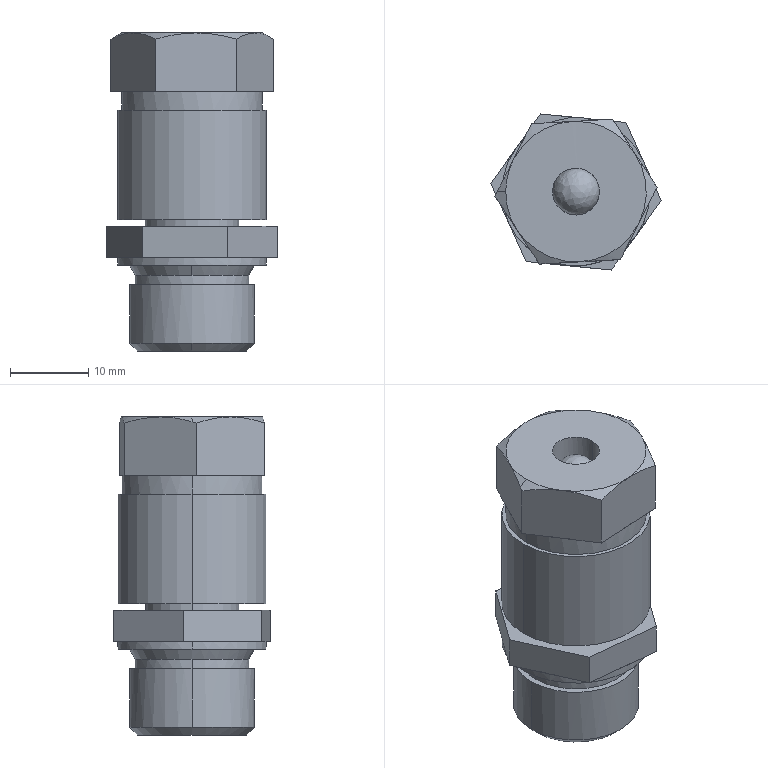Part | SolidWorks | features BaseBody 1 | 1 solid | 75 faces | box 21.831 x 19.996 x 40.743 mm | volume 8193 mm3 | plane 34 | cylinder 26 | cone 13 | spline 2 | commonest cylinder face diameters 4 x4 6 x4 12 x4 14.5 x4 19 x4 5 x2